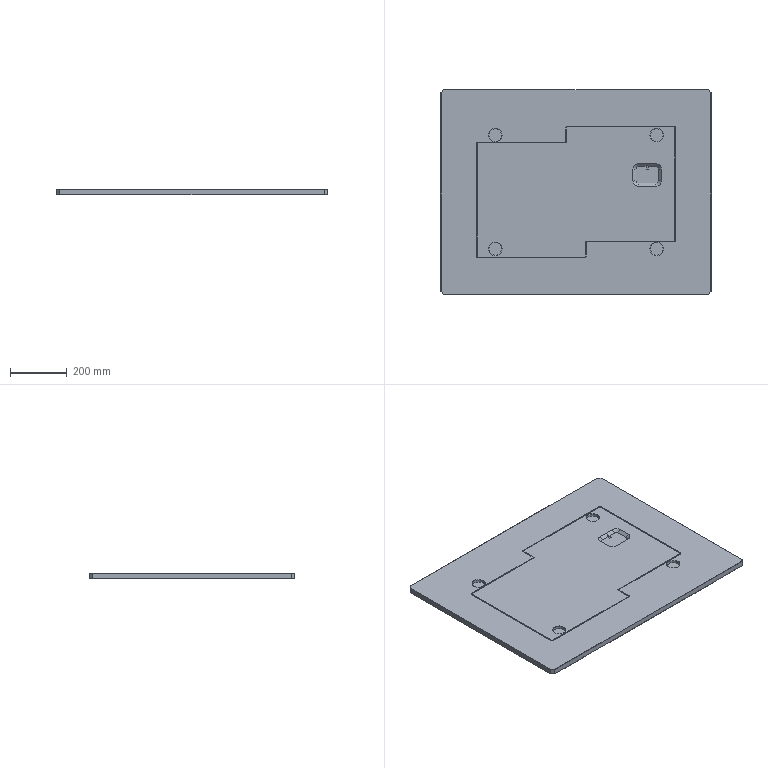Part | STEP file | TJ-DHQM-003-005 | 1 solid | 168 faces | box 950 x 720 x 20 mm | volume 13492361 mm3 | plane 70 | cylinder 56 | cone 42 | commonest cylinder face diameters 4.2 x20 5 x8 45 x8 7.2 x6 12.8 x6 2.2 x2